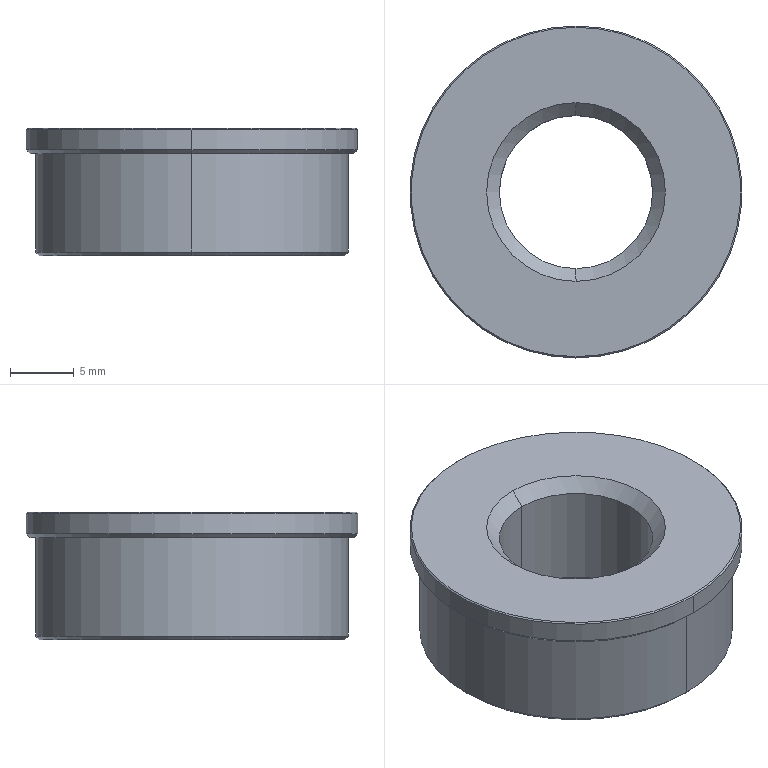Part | SolidWorks | features BaseBody 1 | 1 solid | 19 faces | box 26 x 26 x 10 mm | volume 3655 mm3 | cone 10 | cylinder 6 | plane 3 | commonest cylinder face diameters 12 x2 24.5 x2 26 x2
STEP:
#1=CARTESIAN_POINT('',(513.262,-4.483,244.544));
#2=VERTEX_POINT('',#1);
#3=CARTESIAN_POINT('',(513.262,-16.483,244.544));
#4=VERTEX_POINT('',#3);
#5=CARTESIAN_POINT('',(513.262,-10.483,244.544));
#6=DIRECTION('',(0.000000004,-0.000000009,1.));
#7=DIRECTION('',(-0.4799,-0.8773,-0.000000006));
#8=AXIS2_PLACEMENT_3D('',#5,#6,#7);
#9=CIRCLE('',#8,6.);
#10=EDGE_CURVE('',#2,#4,#9,.T.);
#11=ORIENTED_EDGE('',*,*,#10,.F.);
#12=CARTESIAN_POINT('',(513.262,-3.483,245.544));
#13=VERTEX_POINT('',#12);
#14=CARTESIAN_POINT('',(513.262,-3.483,245.544));
#15=DIRECTION('',(0.000000003,0.7071,0.7071));
#16=VECTOR('',#15,1000.);
#17=LINE('',#14,#16);
#18=EDGE_CURVE('',#2,#13,#17,.T.);
#19=ORIENTED_EDGE('',*,*,#18,.T.);
#20=CARTESIAN_POINT('',(513.262,-17.483,245.544));
#21=VERTEX_POINT('',#20);
#22=CARTESIAN_POINT('',(513.262,-10.483,245.544));
#23=DIRECTION('',(0.000000004,-0.000000009,1.));
#24=DIRECTION('',(0.,-1.,-0.000000009));
#25=AXIS2_PLACEMENT_3D('',#22,#23,#24);
#26=CIRCLE('',#25,7.);
#27=EDGE_CURVE('',#13,#21,#26,.T.);
#28=ORIENTED_EDGE('',*,*,#27,.T.);
#29=CARTESIAN_POINT('',(513.262,-17.483,245.544));
#30=DIRECTION('',(0.000000003,-0.7071,0.7071));
#31=VECTOR('',#30,1000.);
#32=LINE('',#29,#31);
#33=EDGE_CURVE('',#4,#21,#32,.T.);
#34=ORIENTED_EDGE('',*,*,#33,.F.);
#35=EDGE_LOOP('',(#11,#19,#28,#34));
#36=FACE_OUTER_BOUND('',#35,.T.);
#37=CARTESIAN_POINT('',(513.262,-10.483,245.544));
#38=DIRECTION('',(0.000000004,-0.000000009,1.));
#39=DIRECTION('',(0.,-1.,-0.000000009));
#40=AXIS2_PLACEMENT_3D('',#37,#38,#39);
#41=CONICAL_SURFACE('',#40,7.,0.7854);
#42=ADVANCED_FACE('',(#36),#41,.F.);
#43=CARTESIAN_POINT('',(513.262,2.417,245.544));
#44=VERTEX_POINT('',#43);
#45=CARTESIAN_POINT('',(513.262,-23.383,245.544));
#46=VERTEX_POINT('',#45);
#47=CARTESIAN_POINT('',(513.262,-10.483,245.544));
#48=DIRECTION('',(-0.000000004,0.000000009,-1.));
#49=DIRECTION('',(0.,1.,0.000000009));
#50=AXIS2_PLACEMENT_3D('',#47,#48,#49);
#51=CIRCLE('',#50,12.9);
#52=EDGE_CURVE('',#44,#46,#51,.T.);
#53=ORIENTED_EDGE('',*,*,#52,.T.);
#54=CARTESIAN_POINT('',(513.262,-23.483,245.444));
#55=VERTEX_POINT('',#54);
#56=CARTESIAN_POINT('',(513.262,-23.483,245.444));
#57=DIRECTION('',(-0.000000003,-0.7071,-0.7071));
#58=VECTOR('',#57,1000.);
#59=LINE('',#56,#58);
#60=EDGE_CURVE('',#46,#55,#59,.T.);
#61=ORIENTED_EDGE('',*,*,#60,.T.);
#62=CARTESIAN_POINT('',(513.262,2.517,245.444));
#63=VERTEX_POINT('',#62);
#64=CARTESIAN_POINT('',(513.262,-10.483,245.444));
#65=DIRECTION('',(0.000000004,-0.000000009,1.));
#66=DIRECTION('',(-0.4799,-0.8773,-0.000000006));
#67=AXIS2_PLACEMENT_3D('',#64,#65,#66);
#68=CIRCLE('',#67,13.);
#69=EDGE_CURVE('',#55,#63,#68,.T.);
#70=ORIENTED_EDGE('',*,*,#69,.T.);
#71=CARTESIAN_POINT('',(513.262,2.517,245.444));
#72=DIRECTION('',(-0.000000003,0.7071,-0.7071));
#73=VECTOR('',#72,1000.);
#74=LINE('',#71,#73);
#75=EDGE_CURVE('',#44,#63,#74,.T.);
#76=ORIENTED_EDGE('',*,*,#75,.F.);
#77=EDGE_LOOP('',(#53,#61,#70,#76));
#78=FACE_OUTER_BOUND('',#77,.T.);
#79=CARTESIAN_POINT('',(513.262,-10.483,245.444));
#80=DIRECTION('',(-0.000000004,0.000000009,-1.));
#81=DIRECTION('',(0.,1.,0.000000009));
#82=AXIS2_PLACEMENT_3D('',#79,#80,#81);
#83=CONICAL_SURFACE('',#82,13.,0.7854);
#84=ADVANCED_FACE('',(#78),#83,.T.);
#85=ORIENTED_EDGE('',*,*,#10,.T.);
#86=CARTESIAN_POINT('',(513.262,-16.483,236.544));
#87=VERTEX_POINT('',#86);
#88=CARTESIAN_POINT('',(513.262,-16.483,235.544));
#89=DIRECTION('',(-0.000000004,0.000000009,-1.));
#90=VECTOR('',#89,1000.);
#91=LINE('',#88,#90);
#92=EDGE_CURVE('',#4,#87,#91,.T.);
#93=ORIENTED_EDGE('',*,*,#92,.T.);
#94=CARTESIAN_POINT('',(513.262,-4.483,236.544));
#95=VERTEX_POINT('',#94);
#96=CARTESIAN_POINT('',(513.262,-10.483,236.544));
#97=DIRECTION('',(0.000000004,-0.000000009,1.));
#98=DIRECTION('',(0.,1.,0.000000009));
#99=AXIS2_PLACEMENT_3D('',#96,#97,#98);
#100=CIRCLE('',#99,6.);
#101=EDGE_CURVE('',#95,#87,#100,.T.);
#102=ORIENTED_EDGE('',*,*,#101,.F.);
#103=CARTESIAN_POINT('',(513.262,-4.483,235.544));
#104=DIRECTION('',(-0.000000004,0.000000009,-1.));
#105=VECTOR('',#104,1000.);
#106=LINE('',#103,#105);
#107=EDGE_CURVE('',#2,#95,#106,.T.);
#108=ORIENTED_EDGE('',*,*,#107,.F.);
#109=EDGE_LOOP('',(#85,#93,#102,#108));
#110=FACE_OUTER_BOUND('',#109,.T.);
#111=CARTESIAN_POINT('',(513.262,-10.483,235.544));
#112=DIRECTION('',(-0.000000004,0.000000009,-1.));
#113=DIRECTION('',(0.,1.,0.000000009));
#114=AXIS2_PLACEMENT_3D('',#111,#112,#113);
#115=CYLINDRICAL_SURFACE('',#114,6.);
#116=ADVANCED_FACE('',(#110),#115,.F.);
#117=CARTESIAN_POINT('',(513.262,-23.483,243.844));
#118=VERTEX_POINT('',#117);
#119=CARTESIAN_POINT('',(513.262,2.517,243.844));
#120=VERTEX_POINT('',#119);
#121=CARTESIAN_POINT('',(513.262,-10.483,243.844));
#122=DIRECTION('',(0.000000004,-0.000000009,1.));
#123=DIRECTION('',(0.,-1.,-0.000000009));
#124=AXIS2_PLACEMENT_3D('',#121,#122,#123);
#125=CIRCLE('',#124,13.);
#126=EDGE_CURVE('',#118,#120,#125,.T.);
#127=ORIENTED_EDGE('',*,*,#126,.T.);
#128=CARTESIAN_POINT('',(513.262,2.517,245.544));
#129=DIRECTION('',(0.000000004,-0.000000009,1.));
#130=VECTOR('',#129,1000.);
#131=LINE('',#128,#130);
#132=EDGE_CURVE('',#120,#63,#131,.T.);
#133=ORIENTED_EDGE('',*,*,#132,.T.);
#134=ORIENTED_EDGE('',*,*,#69,.F.);
#135=CARTESIAN_POINT('',(513.262,-23.483,245.544));
#136=DIRECTION('',(0.000000004,-0.000000009,1.));
#137=VECTOR('',#136,1000.);
#138=LINE('',#135,#137);
#139=EDGE_CURVE('',#118,#55,#138,.T.);
#140=ORIENTED_EDGE('',*,*,#139,.F.);
#141=EDGE_LOOP('',(#127,#133,#134,#140));
#142=FACE_OUTER_BOUND('',#141,.T.);
#143=CARTESIAN_POINT('',(513.262,-10.483,245.544));
#144=DIRECTION('',(0.000000004,-0.000000009,1.));
#145=DIRECTION('',(0.,-1.,-0.000000009));
#146=AXIS2_PLACEMENT_3D('',#143,#144,#145);
#147=CYLINDRICAL_SURFACE('',#146,13.);
#148=ADVANCED_FACE('',(#142),#147,.T.);
#149=ORIENTED_EDGE('',*,*,#101,.T.);
#150=CARTESIAN_POINT('',(513.262,-17.483,235.544));
#151=VERTEX_POINT('',#150);
#152=CARTESIAN_POINT('',(513.262,-17.483,235.544));
#153=DIRECTION('',(-0.000000003,-0.7071,-0.7071));
#154=VECTOR('',#153,1000.);
#155=LINE('',#152,#154);
#156=EDGE_CURVE('',#87,#151,#155,.T.);
#157=ORIENTED_EDGE('',*,*,#156,.T.);
#158=CARTESIAN_POINT('',(513.262,-3.483,235.544));
#159=VERTEX_POINT('',#158);
#160=CARTESIAN_POINT('',(513.262,-10.483,235.544));
#161=DIRECTION('',(0.000000004,-0.000000009,1.));
#162=DIRECTION('',(0.,1.,0.000000009));
#163=AXIS2_PLACEMENT_3D('',#160,#161,#162);
#164=CIRCLE('',#163,7.);
#165=EDGE_CURVE('',#159,#151,#164,.T.);
#166=ORIENTED_EDGE('',*,*,#165,.F.);
#167=CARTESIAN_POINT('',(513.262,-3.483,235.544));
#168=DIRECTION('',(-0.000000003,0.7071,-0.7071));
#169=VECTOR('',#168,1000.);
#170=LINE('',#167,#169);
#171=EDGE_CURVE('',#95,#159,#170,.T.);
#172=ORIENTED_EDGE('',*,*,#171,.F.);
#173=EDGE_LOOP('',(#149,#157,#166,#172));
#174=FACE_OUTER_BOUND('',#173,.T.);
#175=CARTESIAN_POINT('',(513.262,-10.483,235.544));
#176=DIRECTION('',(-0.000000004,0.000000009,-1.));
#177=DIRECTION('',(0.,1.,0.000000009));
#178=AXIS2_PLACEMENT_3D('',#175,#176,#177);
#179=CONICAL_SURFACE('',#178,7.,0.7854);
#180=ADVANCED_FACE('',(#174),#179,.F.);
#181=CARTESIAN_POINT('',(513.262,-23.183,243.544));
#182=VERTEX_POINT('',#181);
#183=CARTESIAN_POINT('',(513.262,2.217,243.544));
#184=VERTEX_POINT('',#183);
#185=CARTESIAN_POINT('',(513.262,-10.483,243.544));
#186=DIRECTION('',(0.000000004,-0.000000009,1.));
#187=DIRECTION('',(0.,-1.,-0.000000009));
#188=AXIS2_PLACEMENT_3D('',#185,#186,#187);
#189=CIRCLE('',#188,12.7);
#190=EDGE_CURVE('',#182,#184,#189,.T.);
#191=ORIENTED_EDGE('',*,*,#190,.T.);
#192=CARTESIAN_POINT('',(513.262,2.517,243.844));
#193=DIRECTION('',(0.000000003,0.7071,0.7071));
#194=VECTOR('',#193,1000.);
#195=LINE('',#192,#194);
#196=EDGE_CURVE('',#184,#120,#195,.T.);
#197=ORIENTED_EDGE('',*,*,#196,.T.);
#198=ORIENTED_EDGE('',*,*,#126,.F.);
#199=CARTESIAN_POINT('',(513.262,-23.483,243.844));
#200=DIRECTION('',(0.000000003,-0.7071,0.7071));
#201=VECTOR('',#200,1000.);
#202=LINE('',#199,#201);
#203=EDGE_CURVE('',#182,#118,#202,.T.);
#204=ORIENTED_EDGE('',*,*,#203,.F.);
#205=EDGE_LOOP('',(#191,#197,#198,#204));
#206=FACE_OUTER_BOUND('',#205,.T.);
#207=CARTESIAN_POINT('',(513.262,-10.483,243.844));
#208=DIRECTION('',(0.000000004,-0.000000009,1.));
#209=DIRECTION('',(0.,-1.,-0.000000009));
#210=AXIS2_PLACEMENT_3D('',#207,#208,#209);
#211=CONICAL_SURFACE('',#210,13.,0.7854);
#212=ADVANCED_FACE('',(#206),#211,.T.);
#213=CARTESIAN_POINT('',(513.262,1.467,235.544));
#214=VERTEX_POINT('',#213);
#215=CARTESIAN_POINT('',(513.262,-22.433,235.544));
#216=VERTEX_POINT('',#215);
#217=CARTESIAN_POINT('',(513.262,-10.483,235.544));
#218=DIRECTION('',(-0.000000004,0.000000009,-1.));
#219=DIRECTION('',(0.,-1.,-0.000000009));
#220=AXIS2_PLACEMENT_3D('',#217,#218,#219);
#221=CIRCLE('',#220,11.95);
#222=EDGE_CURVE('',#214,#216,#221,.T.);
#223=ORIENTED_EDGE('',*,*,#222,.F.);
#224=CARTESIAN_POINT('',(513.262,1.767,235.844));
#225=VERTEX_POINT('',#224);
#226=CARTESIAN_POINT('',(513.262,1.767,235.844));
#227=DIRECTION('',(0.000000003,0.7071,0.7071));
#228=VECTOR('',#227,1000.);
#229=LINE('',#226,#228);
#230=EDGE_CURVE('',#214,#225,#229,.T.);
#231=ORIENTED_EDGE('',*,*,#230,.T.);
#232=CARTESIAN_POINT('',(513.262,-22.733,235.844));
#233=VERTEX_POINT('',#232);
#234=CARTESIAN_POINT('',(513.262,-10.483,235.844));
#235=DIRECTION('',(-0.000000004,0.000000009,-1.));
#236=DIRECTION('',(0.4799,0.8773,0.000000006));
#237=AXIS2_PLACEMENT_3D('',#234,#235,#236);
#238=CIRCLE('',#237,12.25);
#239=EDGE_CURVE('',#225,#233,#238,.T.);
#240=ORIENTED_EDGE('',*,*,#239,.T.);
#241=CARTESIAN_POINT('',(513.262,-22.733,235.844));
#242=DIRECTION('',(0.000000003,-0.7071,0.7071));
#243=VECTOR('',#242,1000.);
#244=LINE('',#241,#243);
#245=EDGE_CURVE('',#216,#233,#244,.T.);
#246=ORIENTED_EDGE('',*,*,#245,.F.);
#247=EDGE_LOOP('',(#223,#231,#240,#246));
#248=FACE_OUTER_BOUND('',#247,.T.);
#249=CARTESIAN_POINT('',(513.262,-10.483,235.844));
#250=DIRECTION('',(0.000000004,-0.000000009,1.));
#251=DIRECTION('',(0.,-1.,-0.000000009));
#252=AXIS2_PLACEMENT_3D('',#249,#250,#251);
#253=CONICAL_SURFACE('',#252,12.25,0.7854);
#254=ADVANCED_FACE('',(#248),#253,.T.);
#255=CARTESIAN_POINT('',(513.262,1.767,243.544));
#256=VERTEX_POINT('',#255);
#257=CARTESIAN_POINT('',(513.262,-22.733,243.544));
#258=VERTEX_POINT('',#257);
#259=CARTESIAN_POINT('',(513.262,-10.483,243.544));
#260=DIRECTION('',(-0.000000004,0.000000009,-1.));
#261=DIRECTION('',(0.,1.,0.000000009));
#262=AXIS2_PLACEMENT_3D('',#259,#260,#261);
#263=CIRCLE('',#262,12.25);
#264=EDGE_CURVE('',#256,#258,#263,.T.);
#265=ORIENTED_EDGE('',*,*,#264,.T.);
#266=CARTESIAN_POINT('',(513.262,-22.733,235.544));
#267=DIRECTION('',(-0.000000004,0.000000009,-1.));
#268=VECTOR('',#267,1000.);
#269=LINE('',#266,#268);
#270=EDGE_CURVE('',#258,#233,#269,.T.);
#271=ORIENTED_EDGE('',*,*,#270,.T.);
#272=ORIENTED_EDGE('',*,*,#239,.F.);
#273=CARTESIAN_POINT('',(513.262,1.767,235.544));
#274=DIRECTION('',(-0.000000004,0.000000009,-1.));
#275=VECTOR('',#274,1000.);
#276=LINE('',#273,#275);
#277=EDGE_CURVE('',#256,#225,#276,.T.);
#278=ORIENTED_EDGE('',*,*,#277,.F.);
#279=EDGE_LOOP('',(#265,#271,#272,#278));
#280=FACE_OUTER_BOUND('',#279,.T.);
#281=CARTESIAN_POINT('',(513.262,-10.483,235.544));
#282=DIRECTION('',(-0.000000004,0.000000009,-1.));
#283=DIRECTION('',(0.,1.,0.000000009));
#284=AXIS2_PLACEMENT_3D('',#281,#282,#283);
#285=CYLINDRICAL_SURFACE('',#284,12.25);
#286=ADVANCED_FACE('',(#280),#285,.T.);
#287=CARTESIAN_POINT('',(513.262,-10.483,245.544));
#288=DIRECTION('',(0.000000004,-0.000000009,1.));
#289=DIRECTION('',(0.,-1.,-0.000000009));
#290=AXIS2_PLACEMENT_3D('',#287,#288,#289);
#291=CIRCLE('',#290,7.);
#292=EDGE_CURVE('',#21,#13,#291,.T.);
#293=ORIENTED_EDGE('',*,*,#292,.F.);
#294=ORIENTED_EDGE('',*,*,#27,.F.);
#295=EDGE_LOOP('',(#293,#294));
#296=FACE_BOUND('',#295,.T.);
#297=ORIENTED_EDGE('',*,*,#52,.F.);
#298=CARTESIAN_POINT('',(513.262,-10.483,245.544));
#299=DIRECTION('',(-0.000000004,0.000000009,-1.));
#300=DIRECTION('',(0.,1.,0.000000009));
#301=AXIS2_PLACEMENT_3D('',#298,#299,#300);
#302=CIRCLE('',#301,12.9);
#303=EDGE_CURVE('',#46,#44,#302,.T.);
#304=ORIENTED_EDGE('',*,*,#303,.F.);
#305=EDGE_LOOP('',(#297,#304));
#306=FACE_OUTER_BOUND('',#305,.T.);
#307=CARTESIAN_POINT('',(513.262,-10.483,245.544));
#308=DIRECTION('',(-0.000000004,0.000000009,-1.));
#309=DIRECTION('',(0.,1.,0.000000009));
#310=AXIS2_PLACEMENT_3D('',#307,#308,#309);
#311=PLANE('',#310);
#312=ADVANCED_FACE('',(#296,#306),#311,.F.);
#313=ORIENTED_EDGE('',*,*,#18,.F.);
#314=CARTESIAN_POINT('',(513.262,-10.483,244.544));
#315=DIRECTION('',(0.000000004,-0.000000009,1.));
#316=DIRECTION('',(-0.4799,-0.8773,-0.000000006));
#317=AXIS2_PLACEMENT_3D('',#314,#315,#316);
#318=CIRCLE('',#317,6.);
#319=EDGE_CURVE('',#4,#2,#318,.T.);
#320=ORIENTED_EDGE('',*,*,#319,.F.);
#321=ORIENTED_EDGE('',*,*,#33,.T.);
#322=ORIENTED_EDGE('',*,*,#292,.T.);
#323=EDGE_LOOP('',(#313,#320,#321,#322));
#324=FACE_OUTER_BOUND('',#323,.T.);
#325=CARTESIAN_POINT('',(513.262,-10.483,245.544));
#326=DIRECTION('',(0.000000004,-0.000000009,1.));
#327=DIRECTION('',(0.,-1.,-0.000000009));
#328=AXIS2_PLACEMENT_3D('',#325,#326,#327);
#329=CONICAL_SURFACE('',#328,7.,0.7854);
#330=ADVANCED_FACE('',(#324),#329,.F.);
#331=ORIENTED_EDGE('',*,*,#60,.F.);
#332=ORIENTED_EDGE('',*,*,#303,.T.);
#333=ORIENTED_EDGE('',*,*,#75,.T.);
#334=CARTESIAN_POINT('',(513.262,-10.483,245.444));
#335=DIRECTION('',(0.000000004,-0.000000009,1.));
#336=DIRECTION('',(-0.4799,-0.8773,-0.000000006));
#337=AXIS2_PLACEMENT_3D('',#334,#335,#336);
#338=CIRCLE('',#337,13.);
#339=EDGE_CURVE('',#63,#55,#338,.T.);
#340=ORIENTED_EDGE('',*,*,#339,.T.);
#341=EDGE_LOOP('',(#331,#332,#333,#340));
#342=FACE_OUTER_BOUND('',#341,.T.);
#343=CARTESIAN_POINT('',(513.262,-10.483,245.444));
#344=DIRECTION('',(-0.000000004,0.000000009,-1.));
#345=DIRECTION('',(0.,1.,0.000000009));
#346=AXIS2_PLACEMENT_3D('',#343,#344,#345);
#347=CONICAL_SURFACE('',#346,13.,0.7854);
#348=ADVANCED_FACE('',(#342),#347,.T.);
#349=ORIENTED_EDGE('',*,*,#92,.F.);
#350=ORIENTED_EDGE('',*,*,#319,.T.);
#351=ORIENTED_EDGE('',*,*,#107,.T.);
#352=CARTESIAN_POINT('',(513.262,-10.483,236.544));
#353=DIRECTION('',(0.000000004,-0.000000009,1.));
#354=DIRECTION('',(0.,1.,0.000000009));
#355=AXIS2_PLACEMENT_3D('',#352,#353,#354);
#356=CIRCLE('',#355,6.);
#357=EDGE_CURVE('',#87,#95,#356,.T.);
#358=ORIENTED_EDGE('',*,*,#357,.F.);
#359=EDGE_LOOP('',(#349,#350,#351,#358));
#360=FACE_OUTER_BOUND('',#359,.T.);
#361=CARTESIAN_POINT('',(513.262,-10.483,235.544));
#362=DIRECTION('',(-0.000000004,0.000000009,-1.));
#363=DIRECTION('',(0.,1.,0.000000009));
#364=AXIS2_PLACEMENT_3D('',#361,#362,#363);
#365=CYLINDRICAL_SURFACE('',#364,6.);
#366=ADVANCED_FACE('',(#360),#365,.F.);
#367=ORIENTED_EDGE('',*,*,#132,.F.);
#368=CARTESIAN_POINT('',(513.262,-10.483,243.844));
#369=DIRECTION('',(0.000000004,-0.000000009,1.));
#370=DIRECTION('',(0.,-1.,-0.000000009));
#371=AXIS2_PLACEMENT_3D('',#368,#369,#370);
#372=CIRCLE('',#371,13.);
#373=EDGE_CURVE('',#120,#118,#372,.T.);
#374=ORIENTED_EDGE('',*,*,#373,.T.);
#375=ORIENTED_EDGE('',*,*,#139,.T.);
#376=ORIENTED_EDGE('',*,*,#339,.F.);
#377=EDGE_LOOP('',(#367,#374,#375,#376));
#378=FACE_OUTER_BOUND('',#377,.T.);
#379=CARTESIAN_POINT('',(513.262,-10.483,245.544));
#380=DIRECTION('',(0.000000004,-0.000000009,1.));
#381=DIRECTION('',(0.,-1.,-0.000000009));
#382=AXIS2_PLACEMENT_3D('',#379,#380,#381);
#383=CYLINDRICAL_SURFACE('',#382,13.);
#384=ADVANCED_FACE('',(#378),#383,.T.);
#385=ORIENTED_EDGE('',*,*,#156,.F.);
#386=ORIENTED_EDGE('',*,*,#357,.T.);
#387=ORIENTED_EDGE('',*,*,#171,.T.);
#388=CARTESIAN_POINT('',(513.262,-10.483,235.544));
#389=DIRECTION('',(0.000000004,-0.000000009,1.));
#390=DIRECTION('',(0.,1.,0.000000009));
#391=AXIS2_PLACEMENT_3D('',#388,#389,#390);
#392=CIRCLE('',#391,7.);
#393=EDGE_CURVE('',#151,#159,#392,.T.);
#394=ORIENTED_EDGE('',*,*,#393,.F.);
#395=EDGE_LOOP('',(#385,#386,#387,#394));
#396=FACE_OUTER_BOUND('',#395,.T.);
#397=CARTESIAN_POINT('',(513.262,-10.483,235.544));
#398=DIRECTION('',(-0.000000004,0.000000009,-1.));
#399=DIRECTION('',(0.,1.,0.000000009));
#400=AXIS2_PLACEMENT_3D('',#397,#398,#399);
#401=CONICAL_SURFACE('',#400,7.,0.7854);
#402=ADVANCED_FACE('',(#396),#401,.F.);
#403=ORIENTED_EDGE('',*,*,#196,.F.);
#404=CARTESIAN_POINT('',(513.262,-10.483,243.544));
#405=DIRECTION('',(0.000000004,-0.000000009,1.));
#406=DIRECTION('',(0.,-1.,-0.000000009));
#407=AXIS2_PLACEMENT_3D('',#404,#405,#406);
#408=CIRCLE('',#407,12.7);
#409=EDGE_CURVE('',#184,#182,#408,.T.);
#410=ORIENTED_EDGE('',*,*,#409,.T.);
#411=ORIENTED_EDGE('',*,*,#203,.T.);
#412=ORIENTED_EDGE('',*,*,#373,.F.);
#413=EDGE_LOOP('',(#403,#410,#411,#412));
#414=FACE_OUTER_BOUND('',#413,.T.);
#415=CARTESIAN_POINT('',(513.262,-10.483,243.844));
#416=DIRECTION('',(0.000000004,-0.000000009,1.));
#417=DIRECTION('',(0.,-1.,-0.000000009));
#418=AXIS2_PLACEMENT_3D('',#415,#416,#417);
#419=CONICAL_SURFACE('',#418,13.,0.7854);
#420=ADVANCED_FACE('',(#414),#419,.T.);
#421=ORIENTED_EDGE('',*,*,#165,.T.);
#422=ORIENTED_EDGE('',*,*,#393,.T.);
#423=EDGE_LOOP('',(#421,#422));
#424=FACE_BOUND('',#423,.T.);
#425=CARTESIAN_POINT('',(513.262,-10.483,235.544));
#426=DIRECTION('',(-0.000000004,0.000000009,-1.));
#427=DIRECTION('',(0.,-1.,-0.000000009));
#428=AXIS2_PLACEMENT_3D('',#425,#426,#427);
#429=CIRCLE('',#428,11.95);
#430=EDGE_CURVE('',#216,#214,#429,.T.);
#431=ORIENTED_EDGE('',*,*,#430,.T.);
#432=ORIENTED_EDGE('',*,*,#222,.T.);
#433=EDGE_LOOP('',(#431,#432));
#434=FACE_OUTER_BOUND('',#433,.T.);
#435=CARTESIAN_POINT('',(513.262,-10.483,235.544));
#436=DIRECTION('',(-0.000000004,0.000000009,-1.));
#437=DIRECTION('',(0.,1.,0.000000009));
#438=AXIS2_PLACEMENT_3D('',#435,#436,#437);
#439=PLANE('',#438);
#440=ADVANCED_FACE('',(#424,#434),#439,.T.);
#441=ORIENTED_EDGE('',*,*,#190,.F.);
#442=ORIENTED_EDGE('',*,*,#409,.F.);
#443=EDGE_LOOP('',(#441,#442));
#444=FACE_OUTER_BOUND('',#443,.T.);
#445=ORIENTED_EDGE('',*,*,#264,.F.);
#446=CARTESIAN_POINT('',(513.262,-10.483,243.544));
#447=DIRECTION('',(-0.000000004,0.000000009,-1.));
#448=DIRECTION('',(0.,1.,0.000000009));
#449=AXIS2_PLACEMENT_3D('',#446,#447,#448);
#450=CIRCLE('',#449,12.25);
#451=EDGE_CURVE('',#258,#256,#450,.T.);
#452=ORIENTED_EDGE('',*,*,#451,.F.);
#453=EDGE_LOOP('',(#445,#452));
#454=FACE_BOUND('',#453,.T.);
#455=CARTESIAN_POINT('',(513.813,-9.476,243.544));
#456=DIRECTION('',(0.000000004,-0.000000009,1.));
#457=DIRECTION('',(0.,-1.,-0.000000009));
#458=AXIS2_PLACEMENT_3D('',#455,#456,#457);
#459=PLANE('',#458);
#460=ADVANCED_FACE('',(#444,#454),#459,.F.);
#461=ORIENTED_EDGE('',*,*,#230,.F.);
#462=ORIENTED_EDGE('',*,*,#430,.F.);
#463=ORIENTED_EDGE('',*,*,#245,.T.);
#464=CARTESIAN_POINT('',(513.262,-10.483,235.844));
#465=DIRECTION('',(-0.000000004,0.000000009,-1.));
#466=DIRECTION('',(0.4799,0.8773,0.000000006));
#467=AXIS2_PLACEMENT_3D('',#464,#465,#466);
#468=CIRCLE('',#467,12.25);
#469=EDGE_CURVE('',#233,#225,#468,.T.);
#470=ORIENTED_EDGE('',*,*,#469,.T.);
#471=EDGE_LOOP('',(#461,#462,#463,#470));
#472=FACE_OUTER_BOUND('',#471,.T.);
#473=CARTESIAN_POINT('',(513.262,-10.483,235.844));
#474=DIRECTION('',(0.000000004,-0.000000009,1.));
#475=DIRECTION('',(0.,-1.,-0.000000009));
#476=AXIS2_PLACEMENT_3D('',#473,#474,#475);
#477=CONICAL_SURFACE('',#476,12.25,0.7854);
#478=ADVANCED_FACE('',(#472),#477,.T.);
#479=ORIENTED_EDGE('',*,*,#270,.F.);
#480=ORIENTED_EDGE('',*,*,#451,.T.);
#481=ORIENTED_EDGE('',*,*,#277,.T.);
#482=ORIENTED_EDGE('',*,*,#469,.F.);
#483=EDGE_LOOP('',(#479,#480,#481,#482));
#484=FACE_OUTER_BOUND('',#483,.T.);
#485=CARTESIAN_POINT('',(513.262,-10.483,235.544));
#486=DIRECTION('',(-0.000000004,0.000000009,-1.));
#487=DIRECTION('',(0.,1.,0.000000009));
#488=AXIS2_PLACEMENT_3D('',#485,#486,#487);
#489=CYLINDRICAL_SURFACE('',#488,12.25);
#490=ADVANCED_FACE('',(#484),#489,.T.);
#491=CLOSED_SHELL('',(#42,#84,#116,#148,#180,#212,#254,#286,#312,#330,#348,#366,#384,#402,#420,#440,#460,#478,#490));
#492=MANIFOLD_SOLID_BREP('',#491);
#493=CARTESIAN_POINT('',(0.,0.,0.));
#494=DIRECTION('',(0.,0.,1.));
#495=DIRECTION('',(1.,0.,0.));
#496=AXIS2_PLACEMENT_3D('',#493,#494,#495);
#497=(LENGTH_UNIT()NAMED_UNIT(*)SI_UNIT(.MILLI.,.METRE.));
#498=UNCERTAINTY_MEASURE_WITH_UNIT(LENGTH_MEASURE(0.00001),#497,'','');
#499=(NAMED_UNIT(*)PLANE_ANGLE_UNIT()SI_UNIT($,.RADIAN.));
#500=(NAMED_UNIT(*)SI_UNIT($,.STERADIAN.)SOLID_ANGLE_UNIT());
#501=(GEOMETRIC_REPRESENTATION_CONTEXT(3)GLOBAL_UNCERTAINTY_ASSIGNED_CONTEXT((#498))GLOBAL_UNIT_ASSIGNED_CONTEXT((#497,#499,#500))REPRESENTATION_CONTEXT('',''));
#502=ADVANCED_BREP_SHAPE_REPRESENTATION('',(#492,#496),#501);